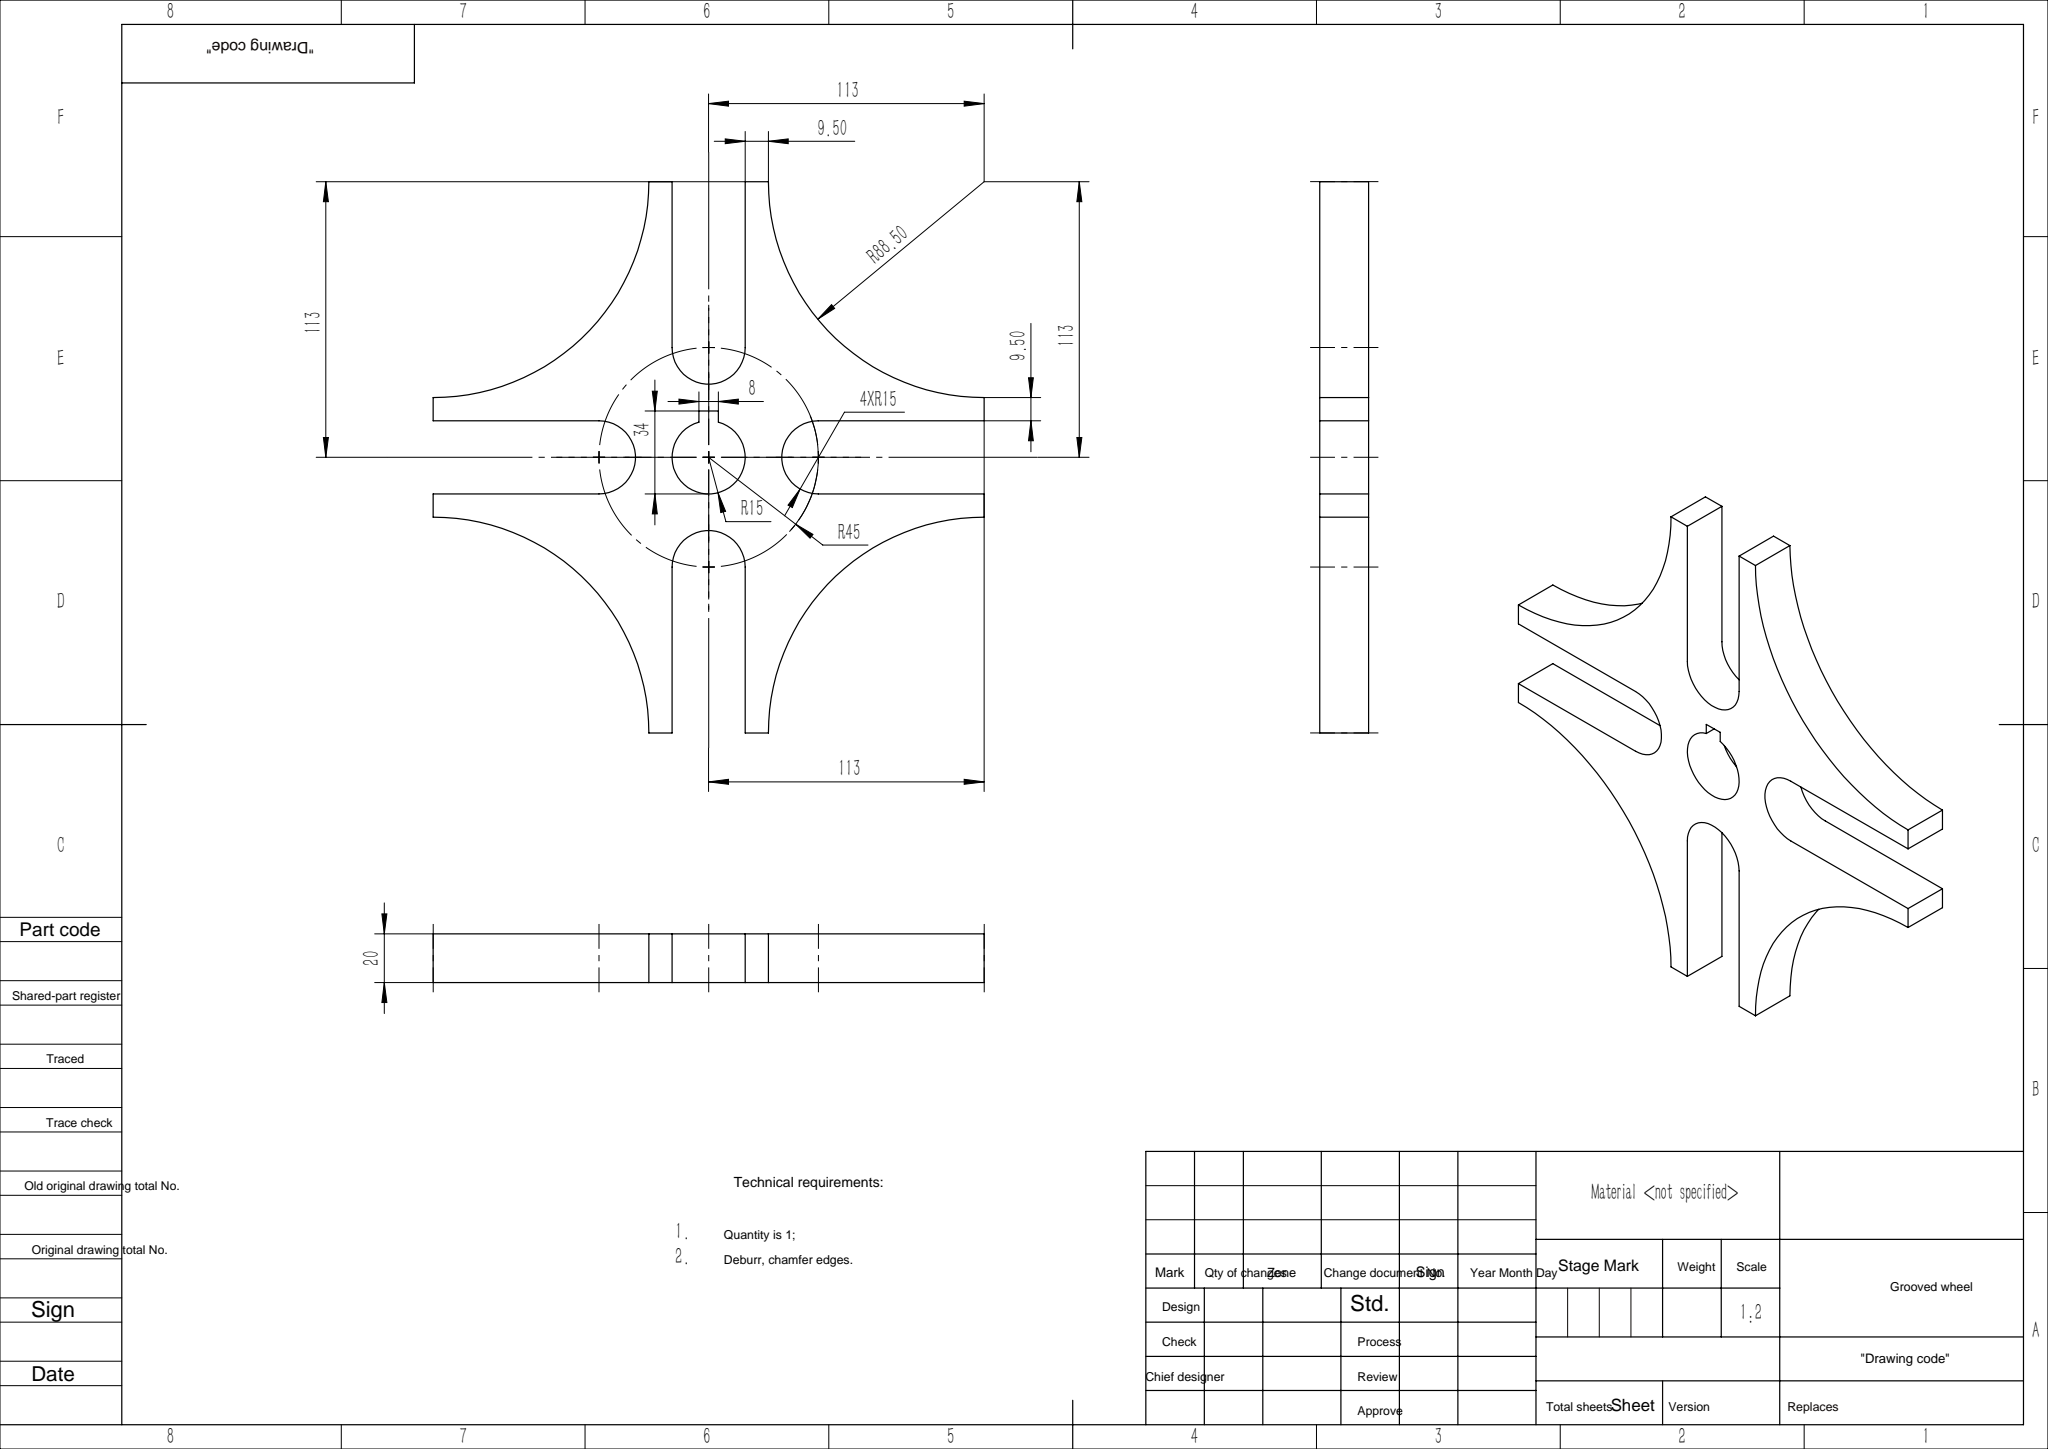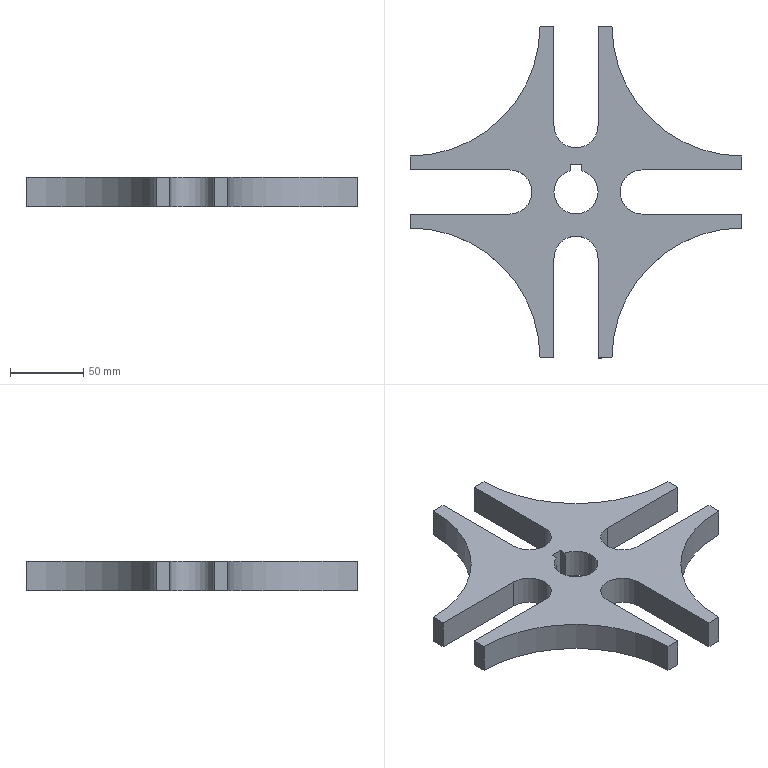Part | SolidWorks | features Extrusion 1, ICE 1 | 1 solid | 33 faces | box 226 x 226 x 20 mm | volume 323125 mm3 | plane 21 | cylinder 12 | commonest cylinder face diameters 30 x8 177 x4
STEP:
#1=CARTESIAN_POINT('',(-15.,0.,0.));
#2=VERTEX_POINT('',#1);
#3=CARTESIAN_POINT('',(15.,0.,0.));
#4=VERTEX_POINT('',#3);
#5=CARTESIAN_POINT('',(0.,0.,0.));
#6=DIRECTION('',(0.,0.,1.));
#7=DIRECTION('',(1.,0.,0.));
#8=AXIS2_PLACEMENT_3D('',#5,#6,#7);
#9=CIRCLE('',#8,15.);
#10=EDGE_CURVE('',#2,#4,#9,.T.);
#11=ORIENTED_EDGE('',*,*,#10,.F.);
#12=CARTESIAN_POINT('',(-15.,0.,20.));
#13=VERTEX_POINT('',#12);
#14=CARTESIAN_POINT('',(-15.,0.,0.));
#15=DIRECTION('',(0.,0.,1.));
#16=VECTOR('',#15,1000.);
#17=LINE('',#14,#16);
#18=EDGE_CURVE('',#2,#13,#17,.T.);
#19=ORIENTED_EDGE('',*,*,#18,.T.);
#20=CARTESIAN_POINT('',(15.,0.,20.));
#21=VERTEX_POINT('',#20);
#22=CARTESIAN_POINT('',(0.,0.,20.));
#23=DIRECTION('',(0.,0.,1.));
#24=DIRECTION('',(1.,0.,0.));
#25=AXIS2_PLACEMENT_3D('',#22,#23,#24);
#26=CIRCLE('',#25,15.);
#27=EDGE_CURVE('',#13,#21,#26,.T.);
#28=ORIENTED_EDGE('',*,*,#27,.T.);
#29=CARTESIAN_POINT('',(15.,0.,0.));
#30=DIRECTION('',(0.,0.,1.));
#31=VECTOR('',#30,1000.);
#32=LINE('',#29,#31);
#33=EDGE_CURVE('',#4,#21,#32,.T.);
#34=ORIENTED_EDGE('',*,*,#33,.F.);
#35=EDGE_LOOP('',(#11,#19,#28,#34));
#36=FACE_OUTER_BOUND('',#35,.T.);
#37=CARTESIAN_POINT('',(0.,0.,0.));
#38=DIRECTION('',(0.,0.,1.));
#39=DIRECTION('',(1.,0.,0.));
#40=AXIS2_PLACEMENT_3D('',#37,#38,#39);
#41=CYLINDRICAL_SURFACE('',#40,15.);
#42=ADVANCED_FACE('',(#36),#41,.F.);
#43=CARTESIAN_POINT('',(4.,14.457,0.));
#44=VERTEX_POINT('',#43);
#45=CARTESIAN_POINT('',(0.,0.,0.));
#46=DIRECTION('',(0.,0.,1.));
#47=DIRECTION('',(1.,0.,0.));
#48=AXIS2_PLACEMENT_3D('',#45,#46,#47);
#49=CIRCLE('',#48,15.);
#50=EDGE_CURVE('',#4,#44,#49,.T.);
#51=ORIENTED_EDGE('',*,*,#50,.F.);
#52=ORIENTED_EDGE('',*,*,#33,.T.);
#53=CARTESIAN_POINT('',(4.,14.457,20.));
#54=VERTEX_POINT('',#53);
#55=CARTESIAN_POINT('',(0.,0.,20.));
#56=DIRECTION('',(0.,0.,1.));
#57=DIRECTION('',(1.,0.,0.));
#58=AXIS2_PLACEMENT_3D('',#55,#56,#57);
#59=CIRCLE('',#58,15.);
#60=EDGE_CURVE('',#21,#54,#59,.T.);
#61=ORIENTED_EDGE('',*,*,#60,.T.);
#62=CARTESIAN_POINT('',(4.,14.457,0.));
#63=DIRECTION('',(0.,0.,1.));
#64=VECTOR('',#63,1000.);
#65=LINE('',#62,#64);
#66=EDGE_CURVE('',#44,#54,#65,.T.);
#67=ORIENTED_EDGE('',*,*,#66,.F.);
#68=EDGE_LOOP('',(#51,#52,#61,#67));
#69=FACE_OUTER_BOUND('',#68,.T.);
#70=CARTESIAN_POINT('',(0.,0.,0.));
#71=DIRECTION('',(0.,0.,1.));
#72=DIRECTION('',(1.,0.,0.));
#73=AXIS2_PLACEMENT_3D('',#70,#71,#72);
#74=CYLINDRICAL_SURFACE('',#73,15.);
#75=ADVANCED_FACE('',(#69),#74,.F.);
#76=CARTESIAN_POINT('',(30.,0.,20.));
#77=VERTEX_POINT('',#76);
#78=CARTESIAN_POINT('',(45.,15.,20.));
#79=VERTEX_POINT('',#78);
#80=CARTESIAN_POINT('',(45.,0.,20.));
#81=DIRECTION('',(0.,0.,-1.));
#82=DIRECTION('',(1.,0.,0.));
#83=AXIS2_PLACEMENT_3D('',#80,#81,#82);
#84=CIRCLE('',#83,15.);
#85=EDGE_CURVE('',#77,#79,#84,.T.);
#86=ORIENTED_EDGE('',*,*,#85,.F.);
#87=CARTESIAN_POINT('',(30.,0.,0.));
#88=VERTEX_POINT('',#87);
#89=CARTESIAN_POINT('',(30.,0.,20.));
#90=DIRECTION('',(0.,0.,-1.));
#91=VECTOR('',#90,1000.);
#92=LINE('',#89,#91);
#93=EDGE_CURVE('',#77,#88,#92,.T.);
#94=ORIENTED_EDGE('',*,*,#93,.T.);
#95=CARTESIAN_POINT('',(45.,15.,0.));
#96=VERTEX_POINT('',#95);
#97=CARTESIAN_POINT('',(45.,0.,0.));
#98=DIRECTION('',(0.,0.,-1.));
#99=DIRECTION('',(1.,0.,0.));
#100=AXIS2_PLACEMENT_3D('',#97,#98,#99);
#101=CIRCLE('',#100,15.);
#102=EDGE_CURVE('',#88,#96,#101,.T.);
#103=ORIENTED_EDGE('',*,*,#102,.T.);
#104=CARTESIAN_POINT('',(45.,15.,20.));
#105=DIRECTION('',(0.,0.,-1.));
#106=VECTOR('',#105,1000.);
#107=LINE('',#104,#106);
#108=EDGE_CURVE('',#79,#96,#107,.T.);
#109=ORIENTED_EDGE('',*,*,#108,.F.);
#110=EDGE_LOOP('',(#86,#94,#103,#109));
#111=FACE_OUTER_BOUND('',#110,.T.);
#112=CARTESIAN_POINT('',(45.,0.,20.));
#113=DIRECTION('',(0.,0.,-1.));
#114=DIRECTION('',(-1.,0.,0.));
#115=AXIS2_PLACEMENT_3D('',#112,#113,#114);
#116=CYLINDRICAL_SURFACE('',#115,15.);
#117=ADVANCED_FACE('',(#111),#116,.F.);
#118=CARTESIAN_POINT('',(-15.,45.,0.));
#119=VERTEX_POINT('',#118);
#120=CARTESIAN_POINT('',(-15.,113.,0.));
#121=VERTEX_POINT('',#120);
#122=CARTESIAN_POINT('',(-15.,45.,0.));
#123=DIRECTION('',(0.,1.,0.));
#124=VECTOR('',#123,1000.);
#125=LINE('',#122,#124);
#126=EDGE_CURVE('',#119,#121,#125,.T.);
#127=ORIENTED_EDGE('',*,*,#126,.T.);
#128=CARTESIAN_POINT('',(-15.,113.,20.));
#129=VERTEX_POINT('',#128);
#130=CARTESIAN_POINT('',(-15.,113.,20.));
#131=DIRECTION('',(0.,0.,-1.));
#132=VECTOR('',#131,1000.);
#133=LINE('',#130,#132);
#134=EDGE_CURVE('',#129,#121,#133,.T.);
#135=ORIENTED_EDGE('',*,*,#134,.F.);
#136=CARTESIAN_POINT('',(-15.,45.,20.));
#137=VERTEX_POINT('',#136);
#138=CARTESIAN_POINT('',(-15.,45.,20.));
#139=DIRECTION('',(0.,1.,0.));
#140=VECTOR('',#139,1000.);
#141=LINE('',#138,#140);
#142=EDGE_CURVE('',#137,#129,#141,.T.);
#143=ORIENTED_EDGE('',*,*,#142,.F.);
#144=CARTESIAN_POINT('',(-15.,45.,20.));
#145=DIRECTION('',(0.,0.,-1.));
#146=VECTOR('',#145,1000.);
#147=LINE('',#144,#146);
#148=EDGE_CURVE('',#137,#119,#147,.T.);
#149=ORIENTED_EDGE('',*,*,#148,.T.);
#150=EDGE_LOOP('',(#127,#135,#143,#149));
#151=FACE_OUTER_BOUND('',#150,.T.);
#152=CARTESIAN_POINT('',(-15.,45.,20.));
#153=DIRECTION('',(-1.,0.,0.));
#154=DIRECTION('',(0.,-1.,0.));
#155=AXIS2_PLACEMENT_3D('',#152,#153,#154);
#156=PLANE('',#155);
#157=ADVANCED_FACE('',(#151),#156,.F.);
#158=CARTESIAN_POINT('',(-24.5,113.,0.));
#159=VERTEX_POINT('',#158);
#160=CARTESIAN_POINT('',(-24.5,113.,0.));
#161=DIRECTION('',(-1.,0.,0.));
#162=VECTOR('',#161,1000.);
#163=LINE('',#160,#162);
#164=EDGE_CURVE('',#121,#159,#163,.T.);
#165=ORIENTED_EDGE('',*,*,#164,.T.);
#166=CARTESIAN_POINT('',(-24.5,113.,20.));
#167=VERTEX_POINT('',#166);
#168=CARTESIAN_POINT('',(-24.5,113.,20.));
#169=DIRECTION('',(0.,0.,-1.));
#170=VECTOR('',#169,1000.);
#171=LINE('',#168,#170);
#172=EDGE_CURVE('',#167,#159,#171,.T.);
#173=ORIENTED_EDGE('',*,*,#172,.F.);
#174=CARTESIAN_POINT('',(-24.5,113.,20.));
#175=DIRECTION('',(-1.,0.,0.));
#176=VECTOR('',#175,1000.);
#177=LINE('',#174,#176);
#178=EDGE_CURVE('',#129,#167,#177,.T.);
#179=ORIENTED_EDGE('',*,*,#178,.F.);
#180=ORIENTED_EDGE('',*,*,#134,.T.);
#181=EDGE_LOOP('',(#165,#173,#179,#180));
#182=FACE_OUTER_BOUND('',#181,.T.);
#183=CARTESIAN_POINT('',(-24.5,113.,20.));
#184=DIRECTION('',(0.,-1.,0.));
#185=DIRECTION('',(1.,0.,0.));
#186=AXIS2_PLACEMENT_3D('',#183,#184,#185);
#187=PLANE('',#186);
#188=ADVANCED_FACE('',(#182),#187,.F.);
#189=CARTESIAN_POINT('',(-113.,24.5,0.));
#190=VERTEX_POINT('',#189);
#191=CARTESIAN_POINT('',(-113.,113.,0.));
#192=DIRECTION('',(0.,0.,-1.));
#193=DIRECTION('',(1.,0.,0.));
#194=AXIS2_PLACEMENT_3D('',#191,#192,#193);
#195=CIRCLE('',#194,88.5);
#196=EDGE_CURVE('',#159,#190,#195,.T.);
#197=ORIENTED_EDGE('',*,*,#196,.T.);
#198=CARTESIAN_POINT('',(-113.,24.5,20.));
#199=VERTEX_POINT('',#198);
#200=CARTESIAN_POINT('',(-113.,24.5,20.));
#201=DIRECTION('',(0.,0.,-1.));
#202=VECTOR('',#201,1000.);
#203=LINE('',#200,#202);
#204=EDGE_CURVE('',#199,#190,#203,.T.);
#205=ORIENTED_EDGE('',*,*,#204,.F.);
#206=CARTESIAN_POINT('',(-113.,113.,20.));
#207=DIRECTION('',(0.,0.,-1.));
#208=DIRECTION('',(1.,0.,0.));
#209=AXIS2_PLACEMENT_3D('',#206,#207,#208);
#210=CIRCLE('',#209,88.5);
#211=EDGE_CURVE('',#167,#199,#210,.T.);
#212=ORIENTED_EDGE('',*,*,#211,.F.);
#213=ORIENTED_EDGE('',*,*,#172,.T.);
#214=EDGE_LOOP('',(#197,#205,#212,#213));
#215=FACE_OUTER_BOUND('',#214,.T.);
#216=CARTESIAN_POINT('',(-113.,113.,20.));
#217=DIRECTION('',(0.,0.,-1.));
#218=DIRECTION('',(-1.,0.,0.));
#219=AXIS2_PLACEMENT_3D('',#216,#217,#218);
#220=CYLINDRICAL_SURFACE('',#219,88.5);
#221=ADVANCED_FACE('',(#215),#220,.F.);
#222=CARTESIAN_POINT('',(-113.,15.,0.));
#223=VERTEX_POINT('',#222);
#224=CARTESIAN_POINT('',(-113.,15.,0.));
#225=DIRECTION('',(0.,-1.,0.));
#226=VECTOR('',#225,1000.);
#227=LINE('',#224,#226);
#228=EDGE_CURVE('',#190,#223,#227,.T.);
#229=ORIENTED_EDGE('',*,*,#228,.T.);
#230=CARTESIAN_POINT('',(-113.,15.,20.));
#231=VERTEX_POINT('',#230);
#232=CARTESIAN_POINT('',(-113.,15.,20.));
#233=DIRECTION('',(0.,0.,-1.));
#234=VECTOR('',#233,1000.);
#235=LINE('',#232,#234);
#236=EDGE_CURVE('',#231,#223,#235,.T.);
#237=ORIENTED_EDGE('',*,*,#236,.F.);
#238=CARTESIAN_POINT('',(-113.,15.,20.));
#239=DIRECTION('',(0.,-1.,0.));
#240=VECTOR('',#239,1000.);
#241=LINE('',#238,#240);
#242=EDGE_CURVE('',#199,#231,#241,.T.);
#243=ORIENTED_EDGE('',*,*,#242,.F.);
#244=ORIENTED_EDGE('',*,*,#204,.T.);
#245=EDGE_LOOP('',(#229,#237,#243,#244));
#246=FACE_OUTER_BOUND('',#245,.T.);
#247=CARTESIAN_POINT('',(-113.,15.,20.));
#248=DIRECTION('',(1.,0.,0.));
#249=DIRECTION('',(0.,1.,0.));
#250=AXIS2_PLACEMENT_3D('',#247,#248,#249);
#251=PLANE('',#250);
#252=ADVANCED_FACE('',(#246),#251,.F.);
#253=CARTESIAN_POINT('',(-45.,15.,0.));
#254=VERTEX_POINT('',#253);
#255=CARTESIAN_POINT('',(-113.,15.,0.));
#256=DIRECTION('',(1.,0.,0.));
#257=VECTOR('',#256,1000.);
#258=LINE('',#255,#257);
#259=EDGE_CURVE('',#223,#254,#258,.T.);
#260=ORIENTED_EDGE('',*,*,#259,.T.);
#261=CARTESIAN_POINT('',(-45.,15.,20.));
#262=VERTEX_POINT('',#261);
#263=CARTESIAN_POINT('',(-45.,15.,20.));
#264=DIRECTION('',(0.,0.,-1.));
#265=VECTOR('',#264,1000.);
#266=LINE('',#263,#265);
#267=EDGE_CURVE('',#262,#254,#266,.T.);
#268=ORIENTED_EDGE('',*,*,#267,.F.);
#269=CARTESIAN_POINT('',(-113.,15.,20.));
#270=DIRECTION('',(1.,0.,0.));
#271=VECTOR('',#270,1000.);
#272=LINE('',#269,#271);
#273=EDGE_CURVE('',#231,#262,#272,.T.);
#274=ORIENTED_EDGE('',*,*,#273,.F.);
#275=ORIENTED_EDGE('',*,*,#236,.T.);
#276=EDGE_LOOP('',(#260,#268,#274,#275));
#277=FACE_OUTER_BOUND('',#276,.T.);
#278=CARTESIAN_POINT('',(-113.,15.,20.));
#279=DIRECTION('',(0.,1.,0.));
#280=DIRECTION('',(-1.,0.,0.));
#281=AXIS2_PLACEMENT_3D('',#278,#279,#280);
#282=PLANE('',#281);
#283=ADVANCED_FACE('',(#277),#282,.F.);
#284=CARTESIAN_POINT('',(-45.,-15.,0.));
#285=VERTEX_POINT('',#284);
#286=CARTESIAN_POINT('',(-45.,0.,0.));
#287=DIRECTION('',(0.,0.,-1.));
#288=DIRECTION('',(1.,0.,0.));
#289=AXIS2_PLACEMENT_3D('',#286,#287,#288);
#290=CIRCLE('',#289,15.);
#291=EDGE_CURVE('',#254,#285,#290,.T.);
#292=ORIENTED_EDGE('',*,*,#291,.T.);
#293=CARTESIAN_POINT('',(-45.,-15.,20.));
#294=VERTEX_POINT('',#293);
#295=CARTESIAN_POINT('',(-45.,-15.,20.));
#296=DIRECTION('',(0.,0.,-1.));
#297=VECTOR('',#296,1000.);
#298=LINE('',#295,#297);
#299=EDGE_CURVE('',#294,#285,#298,.T.);
#300=ORIENTED_EDGE('',*,*,#299,.F.);
#301=CARTESIAN_POINT('',(-45.,0.,20.));
#302=DIRECTION('',(0.,0.,-1.));
#303=DIRECTION('',(1.,0.,0.));
#304=AXIS2_PLACEMENT_3D('',#301,#302,#303);
#305=CIRCLE('',#304,15.);
#306=EDGE_CURVE('',#262,#294,#305,.T.);
#307=ORIENTED_EDGE('',*,*,#306,.F.);
#308=ORIENTED_EDGE('',*,*,#267,.T.);
#309=EDGE_LOOP('',(#292,#300,#307,#308));
#310=FACE_OUTER_BOUND('',#309,.T.);
#311=CARTESIAN_POINT('',(-45.,0.,20.));
#312=DIRECTION('',(0.,0.,-1.));
#313=DIRECTION('',(-1.,0.,0.));
#314=AXIS2_PLACEMENT_3D('',#311,#312,#313);
#315=CYLINDRICAL_SURFACE('',#314,15.);
#316=ADVANCED_FACE('',(#310),#315,.F.);
#317=CARTESIAN_POINT('',(-113.,-15.,0.));
#318=VERTEX_POINT('',#317);
#319=CARTESIAN_POINT('',(-45.,-15.,0.));
#320=DIRECTION('',(-1.,0.,0.));
#321=VECTOR('',#320,1000.);
#322=LINE('',#319,#321);
#323=EDGE_CURVE('',#285,#318,#322,.T.);
#324=ORIENTED_EDGE('',*,*,#323,.T.);
#325=CARTESIAN_POINT('',(-113.,-15.,20.));
#326=VERTEX_POINT('',#325);
#327=CARTESIAN_POINT('',(-113.,-15.,20.));
#328=DIRECTION('',(0.,0.,-1.));
#329=VECTOR('',#328,1000.);
#330=LINE('',#327,#329);
#331=EDGE_CURVE('',#326,#318,#330,.T.);
#332=ORIENTED_EDGE('',*,*,#331,.F.);
#333=CARTESIAN_POINT('',(-45.,-15.,20.));
#334=DIRECTION('',(-1.,0.,0.));
#335=VECTOR('',#334,1000.);
#336=LINE('',#333,#335);
#337=EDGE_CURVE('',#294,#326,#336,.T.);
#338=ORIENTED_EDGE('',*,*,#337,.F.);
#339=ORIENTED_EDGE('',*,*,#299,.T.);
#340=EDGE_LOOP('',(#324,#332,#338,#339));
#341=FACE_OUTER_BOUND('',#340,.T.);
#342=CARTESIAN_POINT('',(-45.,-15.,20.));
#343=DIRECTION('',(0.,-1.,0.));
#344=DIRECTION('',(1.,0.,0.));
#345=AXIS2_PLACEMENT_3D('',#342,#343,#344);
#346=PLANE('',#345);
#347=ADVANCED_FACE('',(#341),#346,.F.);
#348=CARTESIAN_POINT('',(-113.,-24.5,0.));
#349=VERTEX_POINT('',#348);
#350=CARTESIAN_POINT('',(-113.,-24.5,0.));
#351=DIRECTION('',(0.,-1.,0.));
#352=VECTOR('',#351,1000.);
#353=LINE('',#350,#352);
#354=EDGE_CURVE('',#318,#349,#353,.T.);
#355=ORIENTED_EDGE('',*,*,#354,.T.);
#356=CARTESIAN_POINT('',(-113.,-24.5,20.));
#357=VERTEX_POINT('',#356);
#358=CARTESIAN_POINT('',(-113.,-24.5,20.));
#359=DIRECTION('',(0.,0.,-1.));
#360=VECTOR('',#359,1000.);
#361=LINE('',#358,#360);
#362=EDGE_CURVE('',#357,#349,#361,.T.);
#363=ORIENTED_EDGE('',*,*,#362,.F.);
#364=CARTESIAN_POINT('',(-113.,-24.5,20.));
#365=DIRECTION('',(0.,-1.,0.));
#366=VECTOR('',#365,1000.);
#367=LINE('',#364,#366);
#368=EDGE_CURVE('',#326,#357,#367,.T.);
#369=ORIENTED_EDGE('',*,*,#368,.F.);
#370=ORIENTED_EDGE('',*,*,#331,.T.);
#371=EDGE_LOOP('',(#355,#363,#369,#370));
#372=FACE_OUTER_BOUND('',#371,.T.);
#373=CARTESIAN_POINT('',(-113.,-24.5,20.));
#374=DIRECTION('',(1.,0.,0.));
#375=DIRECTION('',(0.,1.,0.));
#376=AXIS2_PLACEMENT_3D('',#373,#374,#375);
#377=PLANE('',#376);
#378=ADVANCED_FACE('',(#372),#377,.F.);
#379=CARTESIAN_POINT('',(-24.5,-113.,0.));
#380=VERTEX_POINT('',#379);
#381=CARTESIAN_POINT('',(-113.,-113.,0.));
#382=DIRECTION('',(0.,0.,-1.));
#383=DIRECTION('',(1.,0.,0.));
#384=AXIS2_PLACEMENT_3D('',#381,#382,#383);
#385=CIRCLE('',#384,88.5);
#386=EDGE_CURVE('',#349,#380,#385,.T.);
#387=ORIENTED_EDGE('',*,*,#386,.T.);
#388=CARTESIAN_POINT('',(-24.5,-113.,20.));
#389=VERTEX_POINT('',#388);
#390=CARTESIAN_POINT('',(-24.5,-113.,20.));
#391=DIRECTION('',(0.,0.,-1.));
#392=VECTOR('',#391,1000.);
#393=LINE('',#390,#392);
#394=EDGE_CURVE('',#389,#380,#393,.T.);
#395=ORIENTED_EDGE('',*,*,#394,.F.);
#396=CARTESIAN_POINT('',(-113.,-113.,20.));
#397=DIRECTION('',(0.,0.,-1.));
#398=DIRECTION('',(1.,0.,0.));
#399=AXIS2_PLACEMENT_3D('',#396,#397,#398);
#400=CIRCLE('',#399,88.5);
#401=EDGE_CURVE('',#357,#389,#400,.T.);
#402=ORIENTED_EDGE('',*,*,#401,.F.);
#403=ORIENTED_EDGE('',*,*,#362,.T.);
#404=EDGE_LOOP('',(#387,#395,#402,#403));
#405=FACE_OUTER_BOUND('',#404,.T.);
#406=CARTESIAN_POINT('',(-113.,-113.,20.));
#407=DIRECTION('',(0.,0.,-1.));
#408=DIRECTION('',(-1.,0.,0.));
#409=AXIS2_PLACEMENT_3D('',#406,#407,#408);
#410=CYLINDRICAL_SURFACE('',#409,88.5);
#411=ADVANCED_FACE('',(#405),#410,.F.);
#412=CARTESIAN_POINT('',(-15.,-113.,0.));
#413=VERTEX_POINT('',#412);
#414=CARTESIAN_POINT('',(-15.,-113.,0.));
#415=DIRECTION('',(1.,0.,0.));
#416=VECTOR('',#415,1000.);
#417=LINE('',#414,#416);
#418=EDGE_CURVE('',#380,#413,#417,.T.);
#419=ORIENTED_EDGE('',*,*,#418,.T.);
#420=CARTESIAN_POINT('',(-15.,-113.,20.));
#421=VERTEX_POINT('',#420);
#422=CARTESIAN_POINT('',(-15.,-113.,20.));
#423=DIRECTION('',(0.,0.,-1.));
#424=VECTOR('',#423,1000.);
#425=LINE('',#422,#424);
#426=EDGE_CURVE('',#421,#413,#425,.T.);
#427=ORIENTED_EDGE('',*,*,#426,.F.);
#428=CARTESIAN_POINT('',(-15.,-113.,20.));
#429=DIRECTION('',(1.,0.,0.));
#430=VECTOR('',#429,1000.);
#431=LINE('',#428,#430);
#432=EDGE_CURVE('',#389,#421,#431,.T.);
#433=ORIENTED_EDGE('',*,*,#432,.F.);
#434=ORIENTED_EDGE('',*,*,#394,.T.);
#435=EDGE_LOOP('',(#419,#427,#433,#434));
#436=FACE_OUTER_BOUND('',#435,.T.);
#437=CARTESIAN_POINT('',(-15.,-113.,20.));
#438=DIRECTION('',(0.,1.,0.));
#439=DIRECTION('',(-1.,0.,0.));
#440=AXIS2_PLACEMENT_3D('',#437,#438,#439);
#441=PLANE('',#440);
#442=ADVANCED_FACE('',(#436),#441,.F.);
#443=CARTESIAN_POINT('',(-15.,-45.,0.));
#444=VERTEX_POINT('',#443);
#445=CARTESIAN_POINT('',(-15.,-113.,0.));
#446=DIRECTION('',(0.,1.,0.));
#447=VECTOR('',#446,1000.);
#448=LINE('',#445,#447);
#449=EDGE_CURVE('',#413,#444,#448,.T.);
#450=ORIENTED_EDGE('',*,*,#449,.T.);
#451=CARTESIAN_POINT('',(-15.,-45.,20.));
#452=VERTEX_POINT('',#451);
#453=CARTESIAN_POINT('',(-15.,-45.,20.));
#454=DIRECTION('',(0.,0.,-1.));
#455=VECTOR('',#454,1000.);
#456=LINE('',#453,#455);
#457=EDGE_CURVE('',#452,#444,#456,.T.);
#458=ORIENTED_EDGE('',*,*,#457,.F.);
#459=CARTESIAN_POINT('',(-15.,-113.,20.));
#460=DIRECTION('',(0.,1.,0.));
#461=VECTOR('',#460,1000.);
#462=LINE('',#459,#461);
#463=EDGE_CURVE('',#421,#452,#462,.T.);
#464=ORIENTED_EDGE('',*,*,#463,.F.);
#465=ORIENTED_EDGE('',*,*,#426,.T.);
#466=EDGE_LOOP('',(#450,#458,#464,#465));
#467=FACE_OUTER_BOUND('',#466,.T.);
#468=CARTESIAN_POINT('',(-15.,-113.,20.));
#469=DIRECTION('',(-1.,0.,0.));
#470=DIRECTION('',(0.,-1.,0.));
#471=AXIS2_PLACEMENT_3D('',#468,#469,#470);
#472=PLANE('',#471);
#473=ADVANCED_FACE('',(#467),#472,.F.);
#474=CARTESIAN_POINT('',(15.,-45.,0.));
#475=VERTEX_POINT('',#474);
#476=CARTESIAN_POINT('',(0.,-45.,0.));
#477=DIRECTION('',(0.,0.,-1.));
#478=DIRECTION('',(1.,0.,0.));
#479=AXIS2_PLACEMENT_3D('',#476,#477,#478);
#480=CIRCLE('',#479,15.);
#481=EDGE_CURVE('',#444,#475,#480,.T.);
#482=ORIENTED_EDGE('',*,*,#481,.T.);
#483=CARTESIAN_POINT('',(15.,-45.,20.));
#484=VERTEX_POINT('',#483);
#485=CARTESIAN_POINT('',(15.,-45.,20.));
#486=DIRECTION('',(0.,0.,-1.));
#487=VECTOR('',#486,1000.);
#488=LINE('',#485,#487);
#489=EDGE_CURVE('',#484,#475,#488,.T.);
#490=ORIENTED_EDGE('',*,*,#489,.F.);
#491=CARTESIAN_POINT('',(0.,-45.,20.));
#492=DIRECTION('',(0.,0.,-1.));
#493=DIRECTION('',(1.,0.,0.));
#494=AXIS2_PLACEMENT_3D('',#491,#492,#493);
#495=CIRCLE('',#494,15.);
#496=EDGE_CURVE('',#452,#484,#495,.T.);
#497=ORIENTED_EDGE('',*,*,#496,.F.);
#498=ORIENTED_EDGE('',*,*,#457,.T.);
#499=EDGE_LOOP('',(#482,#490,#497,#498));
#500=FACE_OUTER_BOUND('',#499,.T.);
#501=CARTESIAN_POINT('',(0.,-45.,20.));
#502=DIRECTION('',(0.,0.,-1.));
#503=DIRECTION('',(-1.,0.,0.));
#504=AXIS2_PLACEMENT_3D('',#501,#502,#503);
#505=CYLINDRICAL_SURFACE('',#504,15.);
#506=ADVANCED_FACE('',(#500),#505,.F.);
#507=CARTESIAN_POINT('',(15.,-113.,0.));
#508=VERTEX_POINT('',#507);
#509=CARTESIAN_POINT('',(15.,-45.,0.));
#510=DIRECTION('',(0.,-1.,0.));
#511=VECTOR('',#510,1000.);
#512=LINE('',#509,#511);
#513=EDGE_CURVE('',#475,#508,#512,.T.);
#514=ORIENTED_EDGE('',*,*,#513,.T.);
#515=CARTESIAN_POINT('',(15.,-113.,20.));
#516=VERTEX_POINT('',#515);
#517=CARTESIAN_POINT('',(15.,-113.,20.));
#518=DIRECTION('',(0.,0.,-1.));
#519=VECTOR('',#518,1000.);
#520=LINE('',#517,#519);
#521=EDGE_CURVE('',#516,#508,#520,.T.);
#522=ORIENTED_EDGE('',*,*,#521,.F.);
#523=CARTESIAN_POINT('',(15.,-45.,20.));
#524=DIRECTION('',(0.,-1.,0.));
#525=VECTOR('',#524,1000.);
#526=LINE('',#523,#525);
#527=EDGE_CURVE('',#484,#516,#526,.T.);
#528=ORIENTED_EDGE('',*,*,#527,.F.);
#529=ORIENTED_EDGE('',*,*,#489,.T.);
#530=EDGE_LOOP('',(#514,#522,#528,#529));
#531=FACE_OUTER_BOUND('',#530,.T.);
#532=CARTESIAN_POINT('',(15.,-45.,20.));
#533=DIRECTION('',(1.,0.,0.));
#534=DIRECTION('',(0.,1.,0.));
#535=AXIS2_PLACEMENT_3D('',#532,#533,#534);
#536=PLANE('',#535);
#537=ADVANCED_FACE('',(#531),#536,.F.);
#538=CARTESIAN_POINT('',(24.5,-113.,0.));
#539=VERTEX_POINT('',#538);
#540=CARTESIAN_POINT('',(24.5,-113.,0.));
#541=DIRECTION('',(1.,0.,0.));
#542=VECTOR('',#541,1000.);
#543=LINE('',#540,#542);
#544=EDGE_CURVE('',#508,#539,#543,.T.);
#545=ORIENTED_EDGE('',*,*,#544,.T.);
#546=CARTESIAN_POINT('',(24.5,-113.,20.));
#547=VERTEX_POINT('',#546);
#548=CARTESIAN_POINT('',(24.5,-113.,20.));
#549=DIRECTION('',(0.,0.,-1.));
#550=VECTOR('',#549,1000.);
#551=LINE('',#548,#550);
#552=EDGE_CURVE('',#547,#539,#551,.T.);
#553=ORIENTED_EDGE('',*,*,#552,.F.);
#554=CARTESIAN_POINT('',(24.5,-113.,20.));
#555=DIRECTION('',(1.,0.,0.));
#556=VECTOR('',#555,1000.);
#557=LINE('',#554,#556);
#558=EDGE_CURVE('',#516,#547,#557,.T.);
#559=ORIENTED_EDGE('',*,*,#558,.F.);
#560=ORIENTED_EDGE('',*,*,#521,.T.);
#561=EDGE_LOOP('',(#545,#553,#559,#560));
#562=FACE_OUTER_BOUND('',#561,.T.);
#563=CARTESIAN_POINT('',(24.5,-113.,20.));
#564=DIRECTION('',(0.,1.,0.));
#565=DIRECTION('',(-1.,0.,0.));
#566=AXIS2_PLACEMENT_3D('',#563,#564,#565);
#567=PLANE('',#566);
#568=ADVANCED_FACE('',(#562),#567,.F.);
#569=CARTESIAN_POINT('',(113.,-24.5,0.));
#570=VERTEX_POINT('',#569);
#571=CARTESIAN_POINT('',(113.,-113.,0.));
#572=DIRECTION('',(0.,0.,-1.));
#573=DIRECTION('',(1.,0.,0.));
#574=AXIS2_PLACEMENT_3D('',#571,#572,#573);
#575=CIRCLE('',#574,88.5);
#576=EDGE_CURVE('',#539,#570,#575,.T.);
#577=ORIENTED_EDGE('',*,*,#576,.T.);
#578=CARTESIAN_POINT('',(113.,-24.5,20.));
#579=VERTEX_POINT('',#578);
#580=CARTESIAN_POINT('',(113.,-24.5,20.));
#581=DIRECTION('',(0.,0.,-1.));
#582=VECTOR('',#581,1000.);
#583=LINE('',#580,#582);
#584=EDGE_CURVE('',#579,#570,#583,.T.);
#585=ORIENTED_EDGE('',*,*,#584,.F.);
#586=CARTESIAN_POINT('',(113.,-113.,20.));
#587=DIRECTION('',(0.,0.,-1.));
#588=DIRECTION('',(1.,0.,0.));
#589=AXIS2_PLACEMENT_3D('',#586,#587,#588);
#590=CIRCLE('',#589,88.5);
#591=EDGE_CURVE('',#547,#579,#590,.T.);
#592=ORIENTED_EDGE('',*,*,#591,.F.);
#593=ORIENTED_EDGE('',*,*,#552,.T.);
#594=EDGE_LOOP('',(#577,#585,#592,#593));
#595=FACE_OUTER_BOUND('',#594,.T.);
#596=CARTESIAN_POINT('',(113.,-113.,20.));
#597=DIRECTION('',(0.,0.,-1.));
#598=DIRECTION('',(-1.,0.,0.));
#599=AXIS2_PLACEMENT_3D('',#596,#597,#598);
#600=CYLINDRICAL_SURFACE('',#599,88.5);
#601=ADVANCED_FACE('',(#595),#600,.F.);
#602=CARTESIAN_POINT('',(113.,-15.,0.));
#603=VERTEX_POINT('',#602);
#604=CARTESIAN_POINT('',(113.,-15.,0.));
#605=DIRECTION('',(0.,1.,0.));
#606=VECTOR('',#605,1000.);
#607=LINE('',#604,#606);
#608=EDGE_CURVE('',#570,#603,#607,.T.);
#609=ORIENTED_EDGE('',*,*,#608,.T.);
#610=CARTESIAN_POINT('',(113.,-15.,20.));
#611=VERTEX_POINT('',#610);
#612=CARTESIAN_POINT('',(113.,-15.,20.));
#613=DIRECTION('',(0.,0.,-1.));
#614=VECTOR('',#613,1000.);
#615=LINE('',#612,#614);
#616=EDGE_CURVE('',#611,#603,#615,.T.);
#617=ORIENTED_EDGE('',*,*,#616,.F.);
#618=CARTESIAN_POINT('',(113.,-15.,20.));
#619=DIRECTION('',(0.,1.,0.));
#620=VECTOR('',#619,1000.);
#621=LINE('',#618,#620);
#622=EDGE_CURVE('',#579,#611,#621,.T.);
#623=ORIENTED_EDGE('',*,*,#622,.F.);
#624=ORIENTED_EDGE('',*,*,#584,.T.);
#625=EDGE_LOOP('',(#609,#617,#623,#624));
#626=FACE_OUTER_BOUND('',#625,.T.);
#627=CARTESIAN_POINT('',(113.,-15.,20.));
#628=DIRECTION('',(-1.,0.,0.));
#629=DIRECTION('',(0.,-1.,0.));
#630=AXIS2_PLACEMENT_3D('',#627,#628,#629);
#631=PLANE('',#630);
#632=ADVANCED_FACE('',(#626),#631,.F.);
#633=CARTESIAN_POINT('',(45.,-15.,0.));
#634=VERTEX_POINT('',#633);
#635=CARTESIAN_POINT('',(113.,-15.,0.));
#636=DIRECTION('',(-1.,0.,0.));
#637=VECTOR('',#636,1000.);
#638=LINE('',#635,#637);
#639=EDGE_CURVE('',#603,#634,#638,.T.);
#640=ORIENTED_EDGE('',*,*,#639,.T.);
#641=CARTESIAN_POINT('',(45.,-15.,20.));
#642=VERTEX_POINT('',#641);
#643=CARTESIAN_POINT('',(45.,-15.,20.));
#644=DIRECTION('',(0.,0.,-1.));
#645=VECTOR('',#644,1000.);
#646=LINE('',#643,#645);
#647=EDGE_CURVE('',#642,#634,#646,.T.);
#648=ORIENTED_EDGE('',*,*,#647,.F.);
#649=CARTESIAN_POINT('',(113.,-15.,20.));
#650=DIRECTION('',(-1.,0.,0.));
#651=VECTOR('',#650,1000.);
#652=LINE('',#649,#651);
#653=EDGE_CURVE('',#611,#642,#652,.T.);
#654=ORIENTED_EDGE('',*,*,#653,.F.);
#655=ORIENTED_EDGE('',*,*,#616,.T.);
#656=EDGE_LOOP('',(#640,#648,#654,#655));
#657=FACE_OUTER_BOUND('',#656,.T.);
#658=CARTESIAN_POINT('',(113.,-15.,20.));
#659=DIRECTION('',(0.,-1.,0.));
#660=DIRECTION('',(1.,0.,0.));
#661=AXIS2_PLACEMENT_3D('',#658,#659,#660);
#662=PLANE('',#661);
#663=ADVANCED_FACE('',(#657),#662,.F.);
#664=ORIENTED_EDGE('',*,*,#93,.F.);
#665=CARTESIAN_POINT('',(45.,0.,20.));
#666=DIRECTION('',(0.,0.,-1.));
#667=DIRECTION('',(1.,0.,0.));
#668=AXIS2_PLACEMENT_3D('',#665,#666,#667);
#669=CIRCLE('',#668,15.);
#670=EDGE_CURVE('',#642,#77,#669,.T.);
#671=ORIENTED_EDGE('',*,*,#670,.F.);
#672=ORIENTED_EDGE('',*,*,#647,.T.);
#673=CARTESIAN_POINT('',(45.,0.,0.));
#674=DIRECTION('',(0.,0.,-1.));
#675=DIRECTION('',(1.,0.,0.));
#676=AXIS2_PLACEMENT_3D('',#673,#674,#675);
#677=CIRCLE('',#676,15.);
#678=EDGE_CURVE('',#634,#88,#677,.T.);
#679=ORIENTED_EDGE('',*,*,#678,.T.);
#680=EDGE_LOOP('',(#664,#671,#672,#679));
#681=FACE_OUTER_BOUND('',#680,.T.);
#682=CARTESIAN_POINT('',(45.,0.,20.));
#683=DIRECTION('',(0.,0.,-1.));
#684=DIRECTION('',(-1.,0.,0.));
#685=AXIS2_PLACEMENT_3D('',#682,#683,#684);
#686=CYLINDRICAL_SURFACE('',#685,15.);
#687=ADVANCED_FACE('',(#681),#686,.F.);
#688=CARTESIAN_POINT('',(113.,15.,0.));
#689=VERTEX_POINT('',#688);
#690=CARTESIAN_POINT('',(45.,15.,0.));
#691=DIRECTION('',(1.,0.,0.));
#692=VECTOR('',#691,1000.);
#693=LINE('',#690,#692);
#694=EDGE_CURVE('',#96,#689,#693,.T.);
#695=ORIENTED_EDGE('',*,*,#694,.T.);
#696=CARTESIAN_POINT('',(113.,15.,20.));
#697=VERTEX_POINT('',#696);
#698=CARTESIAN_POINT('',(113.,15.,20.));
#699=DIRECTION('',(0.,0.,-1.));
#700=VECTOR('',#699,1000.);
#701=LINE('',#698,#700);
#702=EDGE_CURVE('',#697,#689,#701,.T.);
#703=ORIENTED_EDGE('',*,*,#702,.F.);
#704=CARTESIAN_POINT('',(45.,15.,20.));
#705=DIRECTION('',(1.,0.,0.));
#706=VECTOR('',#705,1000.);
#707=LINE('',#704,#706);
#708=EDGE_CURVE('',#79,#697,#707,.T.);
#709=ORIENTED_EDGE('',*,*,#708,.F.);
#710=ORIENTED_EDGE('',*,*,#108,.T.);
#711=EDGE_LOOP('',(#695,#703,#709,#710));
#712=FACE_OUTER_BOUND('',#711,.T.);
#713=CARTESIAN_POINT('',(45.,15.,20.));
#714=DIRECTION('',(0.,1.,0.));
#715=DIRECTION('',(0.,0.,1.));
#716=AXIS2_PLACEMENT_3D('',#713,#714,#715);
#717=PLANE('',#716);
#718=ADVANCED_FACE('',(#712),#717,.F.);
#719=CARTESIAN_POINT('',(113.,24.5,0.));
#720=VERTEX_POINT('',#719);
#721=CARTESIAN_POINT('',(113.,24.5,0.));
#722=DIRECTION('',(0.,1.,0.));
#723=VECTOR('',#722,1000.);
#724=LINE('',#721,#723);
#725=EDGE_CURVE('',#689,#720,#724,.T.);
#726=ORIENTED_EDGE('',*,*,#725,.T.);
#727=CARTESIAN_POINT('',(113.,24.5,20.));
#728=VERTEX_POINT('',#727);
#729=CARTESIAN_POINT('',(113.,24.5,20.));
#730=DIRECTION('',(0.,0.,-1.));
#731=VECTOR('',#730,1000.);
#732=LINE('',#729,#731);
#733=EDGE_CURVE('',#728,#720,#732,.T.);
#734=ORIENTED_EDGE('',*,*,#733,.F.);
#735=CARTESIAN_POINT('',(113.,24.5,20.));
#736=DIRECTION('',(0.,1.,0.));
#737=VECTOR('',#736,1000.);
#738=LINE('',#735,#737);
#739=EDGE_CURVE('',#697,#728,#738,.T.);
#740=ORIENTED_EDGE('',*,*,#739,.F.);
#741=ORIENTED_EDGE('',*,*,#702,.T.);
#742=EDGE_LOOP('',(#726,#734,#740,#741));
#743=FACE_OUTER_BOUND('',#742,.T.);
#744=CARTESIAN_POINT('',(113.,24.5,20.));
#745=DIRECTION('',(-1.,0.,0.));
#746=DIRECTION('',(0.,0.,1.));
#747=AXIS2_PLACEMENT_3D('',#744,#745,#746);
#748=PLANE('',#747);
#749=ADVANCED_FACE('',(#743),#748,.F.);
#750=CARTESIAN_POINT('',(24.5,113.,0.));
#751=VERTEX_POINT('',#750);
#752=CARTESIAN_POINT('',(113.,113.,0.));
#753=DIRECTION('',(0.,0.,-1.));
#754=DIRECTION('',(1.,0.,0.));
#755=AXIS2_PLACEMENT_3D('',#752,#753,#754);
#756=CIRCLE('',#755,88.5);
#757=EDGE_CURVE('',#720,#751,#756,.T.);
#758=ORIENTED_EDGE('',*,*,#757,.T.);
#759=CARTESIAN_POINT('',(24.5,113.,20.));
#760=VERTEX_POINT('',#759);
#761=CARTESIAN_POINT('',(24.5,113.,20.));
#762=DIRECTION('',(0.,0.,-1.));
#763=VECTOR('',#762,1000.);
#764=LINE('',#761,#763);
#765=EDGE_CURVE('',#760,#751,#764,.T.);
#766=ORIENTED_EDGE('',*,*,#765,.F.);
#767=CARTESIAN_POINT('',(113.,113.,20.));
#768=DIRECTION('',(0.,0.,-1.));
#769=DIRECTION('',(1.,0.,0.));
#770=AXIS2_PLACEMENT_3D('',#767,#768,#769);
#771=CIRCLE('',#770,88.5);
#772=EDGE_CURVE('',#728,#760,#771,.T.);
#773=ORIENTED_EDGE('',*,*,#772,.F.);
#774=ORIENTED_EDGE('',*,*,#733,.T.);
#775=EDGE_LOOP('',(#758,#766,#773,#774));
#776=FACE_OUTER_BOUND('',#775,.T.);
#777=CARTESIAN_POINT('',(113.,113.,20.));
#778=DIRECTION('',(0.,0.,-1.));
#779=DIRECTION('',(-1.,0.,0.));
#780=AXIS2_PLACEMENT_3D('',#777,#778,#779);
#781=CYLINDRICAL_SURFACE('',#780,88.5);
#782=ADVANCED_FACE('',(#776),#781,.F.);
#783=CARTESIAN_POINT('',(15.,113.,0.));
#784=VERTEX_POINT('',#783);
#785=CARTESIAN_POINT('',(15.,113.,0.));
#786=DIRECTION('',(-1.,0.,0.));
#787=VECTOR('',#786,1000.);
#788=LINE('',#785,#787);
#789=EDGE_CURVE('',#751,#784,#788,.T.);
#790=ORIENTED_EDGE('',*,*,#789,.T.);
#791=CARTESIAN_POINT('',(15.,113.,20.));
#792=VERTEX_POINT('',#791);
#793=CARTESIAN_POINT('',(15.,113.,20.));
#794=DIRECTION('',(0.,0.,-1.));
#795=VECTOR('',#794,1000.);
#796=LINE('',#793,#795);
#797=EDGE_CURVE('',#792,#784,#796,.T.);
#798=ORIENTED_EDGE('',*,*,#797,.F.);
#799=CARTESIAN_POINT('',(15.,113.,20.));
#800=DIRECTION('',(-1.,0.,0.));
#801=VECTOR('',#800,1000.);
#802=LINE('',#799,#801);
#803=EDGE_CURVE('',#760,#792,#802,.T.);
#804=ORIENTED_EDGE('',*,*,#803,.F.);
#805=ORIENTED_EDGE('',*,*,#765,.T.);
#806=EDGE_LOOP('',(#790,#798,#804,#805));
#807=FACE_OUTER_BOUND('',#806,.T.);
#808=CARTESIAN_POINT('',(15.,113.,20.));
#809=DIRECTION('',(0.,-1.,0.));
#810=DIRECTION('',(0.,0.,-1.));
#811=AXIS2_PLACEMENT_3D('',#808,#809,#810);
#812=PLANE('',#811);
#813=ADVANCED_FACE('',(#807),#812,.F.);
#814=CARTESIAN_POINT('',(15.,45.,0.));
#815=VERTEX_POINT('',#814);
#816=CARTESIAN_POINT('',(15.,113.,0.));
#817=DIRECTION('',(0.,-1.,0.));
#818=VECTOR('',#817,1000.);
#819=LINE('',#816,#818);
#820=EDGE_CURVE('',#784,#815,#819,.T.);
#821=ORIENTED_EDGE('',*,*,#820,.T.);
#822=CARTESIAN_POINT('',(15.,45.,20.));
#823=VERTEX_POINT('',#822);
#824=CARTESIAN_POINT('',(15.,45.,20.));
#825=DIRECTION('',(0.,0.,-1.));
#826=VECTOR('',#825,1000.);
#827=LINE('',#824,#826);
#828=EDGE_CURVE('',#823,#815,#827,.T.);
#829=ORIENTED_EDGE('',*,*,#828,.F.);
#830=CARTESIAN_POINT('',(15.,113.,20.));
#831=DIRECTION('',(0.,-1.,0.));
#832=VECTOR('',#831,1000.);
#833=LINE('',#830,#832);
#834=EDGE_CURVE('',#792,#823,#833,.T.);
#835=ORIENTED_EDGE('',*,*,#834,.F.);
#836=ORIENTED_EDGE('',*,*,#797,.T.);
#837=EDGE_LOOP('',(#821,#829,#835,#836));
#838=FACE_OUTER_BOUND('',#837,.T.);
#839=CARTESIAN_POINT('',(15.,113.,20.));
#840=DIRECTION('',(1.,0.,0.));
#841=DIRECTION('',(0.,1.,0.));
#842=AXIS2_PLACEMENT_3D('',#839,#840,#841);
#843=PLANE('',#842);
#844=ADVANCED_FACE('',(#838),#843,.F.);
#845=CARTESIAN_POINT('',(0.,45.,0.));
#846=DIRECTION('',(0.,0.,-1.));
#847=DIRECTION('',(1.,0.,0.));
#848=AXIS2_PLACEMENT_3D('',#845,#846,#847);
#849=CIRCLE('',#848,15.);
#850=EDGE_CURVE('',#815,#119,#849,.T.);
#851=ORIENTED_EDGE('',*,*,#850,.T.);
#852=ORIENTED_EDGE('',*,*,#148,.F.);
#853=CARTESIAN_POINT('',(0.,45.,20.));
#854=DIRECTION('',(0.,0.,-1.));
#855=DIRECTION('',(1.,0.,0.));
#856=AXIS2_PLACEMENT_3D('',#853,#854,#855);
#857=CIRCLE('',#856,15.);
#858=EDGE_CURVE('',#823,#137,#857,.T.);
#859=ORIENTED_EDGE('',*,*,#858,.F.);
#860=ORIENTED_EDGE('',*,*,#828,.T.);
#861=EDGE_LOOP('',(#851,#852,#859,#860));
#862=FACE_OUTER_BOUND('',#861,.T.);
#863=CARTESIAN_POINT('',(0.,45.,20.));
#864=DIRECTION('',(0.,0.,-1.));
#865=DIRECTION('',(-1.,0.,0.));
#866=AXIS2_PLACEMENT_3D('',#863,#864,#865);
#867=CYLINDRICAL_SURFACE('',#866,15.);
#868=ADVANCED_FACE('',(#862),#867,.F.);
#869=CARTESIAN_POINT('',(-4.,19.,20.));
#870=VERTEX_POINT('',#869);
#871=CARTESIAN_POINT('',(-4.,14.457,20.));
#872=VERTEX_POINT('',#871);
#873=CARTESIAN_POINT('',(-4.,19.,20.));
#874=DIRECTION('',(0.,-1.,0.));
#875=VECTOR('',#874,1000.);
#876=LINE('',#873,#875);
#877=EDGE_CURVE('',#870,#872,#876,.T.);
#878=ORIENTED_EDGE('',*,*,#877,.F.);
#879=CARTESIAN_POINT('',(4.,19.,20.));
#880=VERTEX_POINT('',#879);
#881=CARTESIAN_POINT('',(-4.,19.,20.));
#882=DIRECTION('',(-1.,0.,0.));
#883=VECTOR('',#882,1000.);
#884=LINE('',#881,#883);
#885=EDGE_CURVE('',#880,#870,#884,.T.);
#886=ORIENTED_EDGE('',*,*,#885,.F.);
#887=CARTESIAN_POINT('',(4.,19.,20.));
#888=DIRECTION('',(0.,1.,0.));
#889=VECTOR('',#888,1000.);
#890=LINE('',#887,#889);
#891=EDGE_CURVE('',#54,#880,#890,.T.);
#892=ORIENTED_EDGE('',*,*,#891,.F.);
#893=ORIENTED_EDGE('',*,*,#60,.F.);
#894=ORIENTED_EDGE('',*,*,#27,.F.);
#895=CARTESIAN_POINT('',(0.,0.,20.));
#896=DIRECTION('',(0.,0.,1.));
#897=DIRECTION('',(1.,0.,0.));
#898=AXIS2_PLACEMENT_3D('',#895,#896,#897);
#899=CIRCLE('',#898,15.);
#900=EDGE_CURVE('',#872,#13,#899,.T.);
#901=ORIENTED_EDGE('',*,*,#900,.F.);
#902=EDGE_LOOP('',(#878,#886,#892,#893,#894,#901));
#903=FACE_BOUND('',#902,.T.);
#904=ORIENTED_EDGE('',*,*,#858,.T.);
#905=ORIENTED_EDGE('',*,*,#142,.T.);
#906=ORIENTED_EDGE('',*,*,#178,.T.);
#907=ORIENTED_EDGE('',*,*,#211,.T.);
#908=ORIENTED_EDGE('',*,*,#242,.T.);
#909=ORIENTED_EDGE('',*,*,#273,.T.);
#910=ORIENTED_EDGE('',*,*,#306,.T.);
#911=ORIENTED_EDGE('',*,*,#337,.T.);
#912=ORIENTED_EDGE('',*,*,#368,.T.);
#913=ORIENTED_EDGE('',*,*,#401,.T.);
#914=ORIENTED_EDGE('',*,*,#432,.T.);
#915=ORIENTED_EDGE('',*,*,#463,.T.);
#916=ORIENTED_EDGE('',*,*,#496,.T.);
#917=ORIENTED_EDGE('',*,*,#527,.T.);
#918=ORIENTED_EDGE('',*,*,#558,.T.);
#919=ORIENTED_EDGE('',*,*,#591,.T.);
#920=ORIENTED_EDGE('',*,*,#622,.T.);
#921=ORIENTED_EDGE('',*,*,#653,.T.);
#922=ORIENTED_EDGE('',*,*,#670,.T.);
#923=ORIENTED_EDGE('',*,*,#85,.T.);
#924=ORIENTED_EDGE('',*,*,#708,.T.);
#925=ORIENTED_EDGE('',*,*,#739,.T.);
#926=ORIENTED_EDGE('',*,*,#772,.T.);
#927=ORIENTED_EDGE('',*,*,#803,.T.);
#928=ORIENTED_EDGE('',*,*,#834,.T.);
#929=EDGE_LOOP('',(#904,#905,#906,#907,#908,#909,#910,#911,#912,#913,#914,#915,#916,#917,#918,#919,#920,#921,#922,#923,#924,#925,#926,#927,#928));
#930=FACE_OUTER_BOUND('',#929,.T.);
#931=CARTESIAN_POINT('',(0.,45.,20.));
#932=DIRECTION('',(0.,0.,1.));
#933=DIRECTION('',(1.,0.,0.));
#934=AXIS2_PLACEMENT_3D('',#931,#932,#933);
#935=PLANE('',#934);
#936=ADVANCED_FACE('',(#903,#930),#935,.T.);
#937=CARTESIAN_POINT('',(4.,19.,0.));
#938=VERTEX_POINT('',#937);
#939=CARTESIAN_POINT('',(-4.,19.,0.));
#940=VERTEX_POINT('',#939);
#941=CARTESIAN_POINT('',(-4.,19.,0.));
#942=DIRECTION('',(-1.,0.,0.));
#943=VECTOR('',#942,1000.);
#944=LINE('',#941,#943);
#945=EDGE_CURVE('',#938,#940,#944,.T.);
#946=ORIENTED_EDGE('',*,*,#945,.T.);
#947=CARTESIAN_POINT('',(-4.,14.457,0.));
#948=VERTEX_POINT('',#947);
#949=CARTESIAN_POINT('',(-4.,19.,0.));
#950=DIRECTION('',(0.,-1.,0.));
#951=VECTOR('',#950,1000.);
#952=LINE('',#949,#951);
#953=EDGE_CURVE('',#940,#948,#952,.T.);
#954=ORIENTED_EDGE('',*,*,#953,.T.);
#955=CARTESIAN_POINT('',(0.,0.,0.));
#956=DIRECTION('',(0.,0.,1.));
#957=DIRECTION('',(1.,0.,0.));
#958=AXIS2_PLACEMENT_3D('',#955,#956,#957);
#959=CIRCLE('',#958,15.);
#960=EDGE_CURVE('',#948,#2,#959,.T.);
#961=ORIENTED_EDGE('',*,*,#960,.T.);
#962=ORIENTED_EDGE('',*,*,#10,.T.);
#963=ORIENTED_EDGE('',*,*,#50,.T.);
#964=CARTESIAN_POINT('',(4.,19.,0.));
#965=DIRECTION('',(0.,1.,0.));
#966=VECTOR('',#965,1000.);
#967=LINE('',#964,#966);
#968=EDGE_CURVE('',#44,#938,#967,.T.);
#969=ORIENTED_EDGE('',*,*,#968,.T.);
#970=EDGE_LOOP('',(#946,#954,#961,#962,#963,#969));
#971=FACE_BOUND('',#970,.T.);
#972=ORIENTED_EDGE('',*,*,#126,.F.);
#973=ORIENTED_EDGE('',*,*,#850,.F.);
#974=ORIENTED_EDGE('',*,*,#820,.F.);
#975=ORIENTED_EDGE('',*,*,#789,.F.);
#976=ORIENTED_EDGE('',*,*,#757,.F.);
#977=ORIENTED_EDGE('',*,*,#725,.F.);
#978=ORIENTED_EDGE('',*,*,#694,.F.);
#979=ORIENTED_EDGE('',*,*,#102,.F.);
#980=ORIENTED_EDGE('',*,*,#678,.F.);
#981=ORIENTED_EDGE('',*,*,#639,.F.);
#982=ORIENTED_EDGE('',*,*,#608,.F.);
#983=ORIENTED_EDGE('',*,*,#576,.F.);
#984=ORIENTED_EDGE('',*,*,#544,.F.);
#985=ORIENTED_EDGE('',*,*,#513,.F.);
#986=ORIENTED_EDGE('',*,*,#481,.F.);
#987=ORIENTED_EDGE('',*,*,#449,.F.);
#988=ORIENTED_EDGE('',*,*,#418,.F.);
#989=ORIENTED_EDGE('',*,*,#386,.F.);
#990=ORIENTED_EDGE('',*,*,#354,.F.);
#991=ORIENTED_EDGE('',*,*,#323,.F.);
#992=ORIENTED_EDGE('',*,*,#291,.F.);
#993=ORIENTED_EDGE('',*,*,#259,.F.);
#994=ORIENTED_EDGE('',*,*,#228,.F.);
#995=ORIENTED_EDGE('',*,*,#196,.F.);
#996=ORIENTED_EDGE('',*,*,#164,.F.);
#997=EDGE_LOOP('',(#972,#973,#974,#975,#976,#977,#978,#979,#980,#981,#982,#983,#984,#985,#986,#987,#988,#989,#990,#991,#992,#993,#994,#995,#996));
#998=FACE_OUTER_BOUND('',#997,.T.);
#999=CARTESIAN_POINT('',(0.,45.,0.));
#1000=DIRECTION('',(0.,0.,1.));
#1001=DIRECTION('',(1.,0.,0.));
#1002=AXIS2_PLACEMENT_3D('',#999,#1000,#1001);
#1003=PLANE('',#1002);
#1004=ADVANCED_FACE('',(#971,#998),#1003,.F.);
#1005=ORIENTED_EDGE('',*,*,#877,.T.);
#1006=CARTESIAN_POINT('',(-4.,14.457,0.));
#1007=DIRECTION('',(0.,0.,1.));
#1008=VECTOR('',#1007,1000.);
#1009=LINE('',#1006,#1008);
#1010=EDGE_CURVE('',#948,#872,#1009,.T.);
#1011=ORIENTED_EDGE('',*,*,#1010,.F.);
#1012=ORIENTED_EDGE('',*,*,#953,.F.);
#1013=CARTESIAN_POINT('',(-4.,19.,0.));
#1014=DIRECTION('',(0.,0.,1.));
#1015=VECTOR('',#1014,1000.);
#1016=LINE('',#1013,#1015);
#1017=EDGE_CURVE('',#940,#870,#1016,.T.);
#1018=ORIENTED_EDGE('',*,*,#1017,.T.);
#1019=EDGE_LOOP('',(#1005,#1011,#1012,#1018));
#1020=FACE_OUTER_BOUND('',#1019,.T.);
#1021=CARTESIAN_POINT('',(-4.,19.,0.));
#1022=DIRECTION('',(-1.,0.,0.));
#1023=DIRECTION('',(0.,-1.,0.));
#1024=AXIS2_PLACEMENT_3D('',#1021,#1022,#1023);
#1025=PLANE('',#1024);
#1026=ADVANCED_FACE('',(#1020),#1025,.F.);
#1027=ORIENTED_EDGE('',*,*,#885,.T.);
#1028=ORIENTED_EDGE('',*,*,#1017,.F.);
#1029=ORIENTED_EDGE('',*,*,#945,.F.);
#1030=CARTESIAN_POINT('',(4.,19.,0.));
#1031=DIRECTION('',(0.,0.,1.));
#1032=VECTOR('',#1031,1000.);
#1033=LINE('',#1030,#1032);
#1034=EDGE_CURVE('',#938,#880,#1033,.T.);
#1035=ORIENTED_EDGE('',*,*,#1034,.T.);
#1036=EDGE_LOOP('',(#1027,#1028,#1029,#1035));
#1037=FACE_OUTER_BOUND('',#1036,.T.);
#1038=CARTESIAN_POINT('',(-4.,19.,0.));
#1039=DIRECTION('',(0.,1.,0.));
#1040=DIRECTION('',(0.,0.,1.));
#1041=AXIS2_PLACEMENT_3D('',#1038,#1039,#1040);
#1042=PLANE('',#1041);
#1043=ADVANCED_FACE('',(#1037),#1042,.F.);
#1044=ORIENTED_EDGE('',*,*,#891,.T.);
#1045=ORIENTED_EDGE('',*,*,#1034,.F.);
#1046=ORIENTED_EDGE('',*,*,#968,.F.);
#1047=ORIENTED_EDGE('',*,*,#66,.T.);
#1048=EDGE_LOOP('',(#1044,#1045,#1046,#1047));
#1049=FACE_OUTER_BOUND('',#1048,.T.);
#1050=CARTESIAN_POINT('',(4.,19.,0.));
#1051=DIRECTION('',(1.,0.,0.));
#1052=DIRECTION('',(0.,1.,0.));
#1053=AXIS2_PLACEMENT_3D('',#1050,#1051,#1052);
#1054=PLANE('',#1053);
#1055=ADVANCED_FACE('',(#1049),#1054,.F.);
#1056=ORIENTED_EDGE('',*,*,#18,.F.);
#1057=ORIENTED_EDGE('',*,*,#960,.F.);
#1058=ORIENTED_EDGE('',*,*,#1010,.T.);
#1059=ORIENTED_EDGE('',*,*,#900,.T.);
#1060=EDGE_LOOP('',(#1056,#1057,#1058,#1059));
#1061=FACE_OUTER_BOUND('',#1060,.T.);
#1062=CARTESIAN_POINT('',(0.,0.,0.));
#1063=DIRECTION('',(0.,0.,1.));
#1064=DIRECTION('',(1.,0.,0.));
#1065=AXIS2_PLACEMENT_3D('',#1062,#1063,#1064);
#1066=CYLINDRICAL_SURFACE('',#1065,15.);
#1067=ADVANCED_FACE('',(#1061),#1066,.F.);
#1068=CLOSED_SHELL('',(#42,#75,#117,#157,#188,#221,#252,#283,#316,#347,#378,#411,#442,#473,#506,#537,#568,#601,#632,#663,#687,#718,#749,#782,#813,#844,#868,#936,#1004,#1026,#1043,#1055,#1067));
#1069=MANIFOLD_SOLID_BREP('',#1068);
#1070=CARTESIAN_POINT('',(0.,0.,0.));
#1071=DIRECTION('',(0.,0.,1.));
#1072=DIRECTION('',(1.,0.,0.));
#1073=AXIS2_PLACEMENT_3D('',#1070,#1071,#1072);
#1074=(LENGTH_UNIT()NAMED_UNIT(*)SI_UNIT(.MILLI.,.METRE.));
#1075=UNCERTAINTY_MEASURE_WITH_UNIT(LENGTH_MEASURE(0.00001),#1074,'','');
#1076=(NAMED_UNIT(*)PLANE_ANGLE_UNIT()SI_UNIT($,.RADIAN.));
#1077=(NAMED_UNIT(*)SI_UNIT($,.STERADIAN.)SOLID_ANGLE_UNIT());
#1078=(GEOMETRIC_REPRESENTATION_CONTEXT(3)GLOBAL_UNCERTAINTY_ASSIGNED_CONTEXT((#1075))GLOBAL_UNIT_ASSIGNED_CONTEXT((#1074,#1076,#1077))REPRESENTATION_CONTEXT('',''));
#1079=ADVANCED_BREP_SHAPE_REPRESENTATION('',(#1069,#1073),#1078);